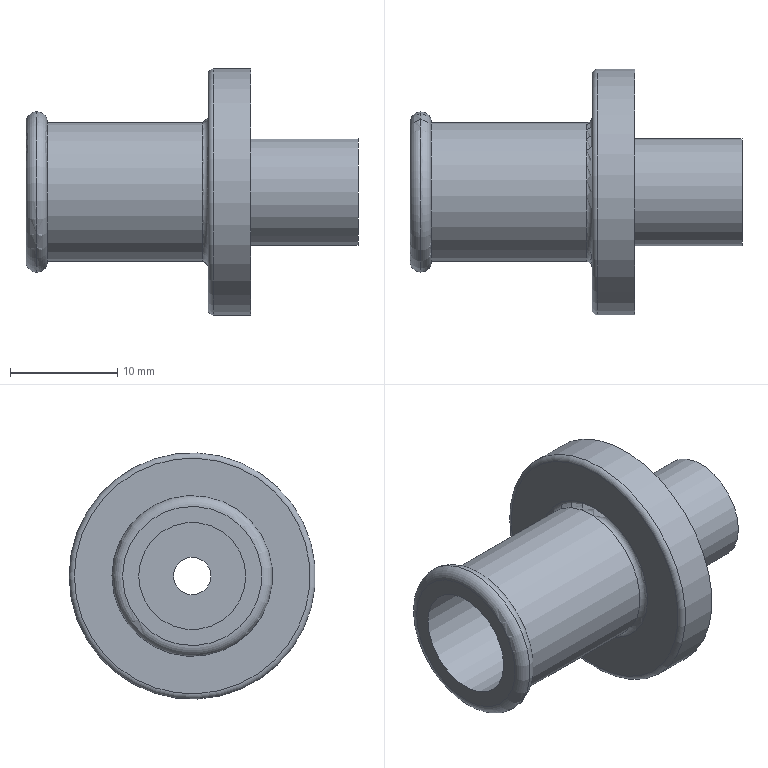Part | STEP file | 1-29.1 | 1 solid | 14 faces | box 31 x 23 x 23 mm | volume 3301 mm3 | cylinder 5 | plane 5 | torus 4 | commonest cylinder face diameters 10 x2 3.5 x1 13 x1 23 x1
STEP:
#1=CARTESIAN_POINT('',(0.,0.,0.));
#2=DIRECTION('',(0.,0.,1.));
#3=DIRECTION('',(1.,0.,0.));
#4=AXIS2_PLACEMENT_3D('',#1,#2,#3);
#5=CARTESIAN_POINT('',(15.,5.,0.));
#6=VERTEX_POINT('',#5);
#7=CARTESIAN_POINT('',(15.,0.,0.));
#8=DIRECTION('',(-1.,0.,0.));
#9=DIRECTION('',(0.,1.,0.));
#10=AXIS2_PLACEMENT_3D('',#7,#8,#9);
#11=CIRCLE('',#10,5.);
#12=CARTESIAN_POINT('',(-2.,0.,0.));
#13=DIRECTION('',(1.,0.,0.));
#14=DIRECTION('',(0.,1.,0.));
#15=AXIS2_PLACEMENT_3D('',#12,#13,#14);
#16=CYLINDRICAL_SURFACE('',#15,5.);
#17=CARTESIAN_POINT('',(6.283,17.));
#18=DIRECTION('',(-1.,0.));
#19=VECTOR('',#18,1.);
#20=LINE('',#17,#19);
#21=(GEOMETRIC_REPRESENTATION_CONTEXT(2)PARAMETRIC_REPRESENTATION_CONTEXT()REPRESENTATION_CONTEXT('',''));
#22=DEFINITIONAL_REPRESENTATION('',(#20),#21);
#23=PCURVE('',#16,#22);
#24=CARTESIAN_POINT('',(15.,-5.75,0.));
#25=DIRECTION('',(1.,0.,0.));
#26=DIRECTION('',(0.,0.,-1.));
#27=AXIS2_PLACEMENT_3D('',#24,#25,#26);
#28=PLANE('',#27);
#29=CARTESIAN_POINT('',(0.,10.75));
#30=CARTESIAN_POINT('',(8.66,10.75));
#31=CARTESIAN_POINT('',(4.33,3.25));
#32=CARTESIAN_POINT('',(0.,-4.25));
#33=CARTESIAN_POINT('',(-4.33,3.25));
#34=CARTESIAN_POINT('',(-8.66,10.75));
#35=CARTESIAN_POINT('',(0.,10.75));
#36=(BOUNDED_CURVE()B_SPLINE_CURVE(2,(#29,#30,#31,#32,#33,#34,#35),.UNSPECIFIED.,.T.,.F.)B_SPLINE_CURVE_WITH_KNOTS((1,2,2,2,2,1),(-2.094,0.,2.094,4.189,6.283,8.378),.UNSPECIFIED.)CURVE()GEOMETRIC_REPRESENTATION_ITEM()RATIONAL_B_SPLINE_CURVE((1.,0.5,1.,0.5,1.,0.5,1.))REPRESENTATION_ITEM(''));
#37=(GEOMETRIC_REPRESENTATION_CONTEXT(2)PARAMETRIC_REPRESENTATION_CONTEXT()REPRESENTATION_CONTEXT('',''));
#38=DEFINITIONAL_REPRESENTATION('',(#36),#37);
#39=PCURVE('',#28,#38);
#40=SURFACE_CURVE('',#11,(#23,#39),.PCURVE_S1.);
#41=EDGE_CURVE('',#6,#6,#40,.T.);
#42=ORIENTED_EDGE('',*,*,#41,.T.);
#43=CARTESIAN_POINT('',(-2.,5.,0.));
#44=VERTEX_POINT('',#43);
#45=CARTESIAN_POINT('',(15.,5.,0.));
#46=DIRECTION('',(-1.,0.,0.));
#47=VECTOR('',#46,1.);
#48=LINE('',#45,#47);
#49=CARTESIAN_POINT('',(0.,17.));
#50=DIRECTION('',(0.,-1.));
#51=VECTOR('',#50,1.);
#52=LINE('',#49,#51);
#53=(GEOMETRIC_REPRESENTATION_CONTEXT(2)PARAMETRIC_REPRESENTATION_CONTEXT()REPRESENTATION_CONTEXT('',''));
#54=DEFINITIONAL_REPRESENTATION('',(#52),#53);
#55=PCURVE('',#16,#54);
#56=CARTESIAN_POINT('',(6.283,17.));
#57=DIRECTION('',(0.,-1.));
#58=VECTOR('',#57,1.);
#59=LINE('',#56,#58);
#60=(GEOMETRIC_REPRESENTATION_CONTEXT(2)PARAMETRIC_REPRESENTATION_CONTEXT()REPRESENTATION_CONTEXT('',''));
#61=DEFINITIONAL_REPRESENTATION('',(#59),#60);
#62=PCURVE('',#16,#61);
#63=SEAM_CURVE('',#48,(#55,#62),.PCURVE_S1.);
#64=EDGE_CURVE('',#6,#44,#63,.T.);
#65=ORIENTED_EDGE('',*,*,#64,.T.);
#66=CARTESIAN_POINT('',(-2.,0.,0.));
#67=DIRECTION('',(-1.,0.,0.));
#68=DIRECTION('',(0.,1.,0.));
#69=AXIS2_PLACEMENT_3D('',#66,#67,#68);
#70=CIRCLE('',#69,5.);
#71=CARTESIAN_POINT('',(6.283,0.));
#72=DIRECTION('',(-1.,0.));
#73=VECTOR('',#72,1.);
#74=LINE('',#71,#73);
#75=(GEOMETRIC_REPRESENTATION_CONTEXT(2)PARAMETRIC_REPRESENTATION_CONTEXT()REPRESENTATION_CONTEXT('',''));
#76=DEFINITIONAL_REPRESENTATION('',(#74),#75);
#77=PCURVE('',#16,#76);
#78=CARTESIAN_POINT('',(-2.,-2.01,0.));
#79=DIRECTION('',(1.,0.,0.));
#80=DIRECTION('',(0.,0.,-1.));
#81=AXIS2_PLACEMENT_3D('',#78,#79,#80);
#82=PLANE('',#81);
#83=CARTESIAN_POINT('',(0.,7.01));
#84=CARTESIAN_POINT('',(8.66,7.01));
#85=CARTESIAN_POINT('',(4.33,-0.4904));
#86=CARTESIAN_POINT('',(0.,-7.99));
#87=CARTESIAN_POINT('',(-4.33,-0.4904));
#88=CARTESIAN_POINT('',(-8.66,7.01));
#89=CARTESIAN_POINT('',(0.,7.01));
#90=(BOUNDED_CURVE()B_SPLINE_CURVE(2,(#83,#84,#85,#86,#87,#88,#89),.UNSPECIFIED.,.T.,.F.)B_SPLINE_CURVE_WITH_KNOTS((1,2,2,2,2,1),(-2.094,0.,2.094,4.189,6.283,8.378),.UNSPECIFIED.)CURVE()GEOMETRIC_REPRESENTATION_ITEM()RATIONAL_B_SPLINE_CURVE((1.,0.5,1.,0.5,1.,0.5,1.))REPRESENTATION_ITEM(''));
#91=(GEOMETRIC_REPRESENTATION_CONTEXT(2)PARAMETRIC_REPRESENTATION_CONTEXT()REPRESENTATION_CONTEXT('',''));
#92=DEFINITIONAL_REPRESENTATION('',(#90),#91);
#93=PCURVE('',#82,#92);
#94=SURFACE_CURVE('',#70,(#77,#93),.PCURVE_S1.);
#95=EDGE_CURVE('',#44,#44,#94,.T.);
#96=ORIENTED_EDGE('',*,*,#95,.F.);
#97=ORIENTED_EDGE('',*,*,#64,.F.);
#98=EDGE_LOOP('',(#42,#65,#96,#97));
#99=FACE_BOUND('',#98,.F.);
#100=ADVANCED_FACE('',(#99),#16,.F.);
#101=CARTESIAN_POINT('',(19.,11.5,0.));
#102=VERTEX_POINT('',#101);
#103=CARTESIAN_POINT('',(19.,0.,0.));
#104=DIRECTION('',(1.,0.,0.));
#105=DIRECTION('',(0.,1.,0.));
#106=AXIS2_PLACEMENT_3D('',#103,#104,#105);
#107=CIRCLE('',#106,11.5);
#108=CARTESIAN_POINT('',(19.,-3.081,0.));
#109=DIRECTION('',(1.,0.,0.));
#110=DIRECTION('',(0.,0.,-1.));
#111=AXIS2_PLACEMENT_3D('',#108,#109,#110);
#112=PLANE('',#111);
#113=CARTESIAN_POINT('',(0.,3.081));
#114=DIRECTION('',(0.,1.));
#115=AXIS2_PLACEMENT_2D('',#113,#114);
#116=CIRCLE('',#115,11.5);
#117=(GEOMETRIC_REPRESENTATION_CONTEXT(2)PARAMETRIC_REPRESENTATION_CONTEXT()REPRESENTATION_CONTEXT('',''));
#118=DEFINITIONAL_REPRESENTATION('',(#116),#117);
#119=PCURVE('',#112,#118);
#120=CARTESIAN_POINT('',(15.,0.,0.));
#121=DIRECTION('',(1.,0.,0.));
#122=DIRECTION('',(0.,1.,0.));
#123=AXIS2_PLACEMENT_3D('',#120,#121,#122);
#124=CYLINDRICAL_SURFACE('',#123,11.5);
#125=CARTESIAN_POINT('',(0.,4.));
#126=DIRECTION('',(1.,0.));
#127=VECTOR('',#126,1.);
#128=LINE('',#125,#127);
#129=(GEOMETRIC_REPRESENTATION_CONTEXT(2)PARAMETRIC_REPRESENTATION_CONTEXT()REPRESENTATION_CONTEXT('',''));
#130=DEFINITIONAL_REPRESENTATION('',(#128),#129);
#131=PCURVE('',#124,#130);
#132=SURFACE_CURVE('',#107,(#119,#131),.PCURVE_S1.);
#133=EDGE_CURVE('',#102,#102,#132,.T.);
#134=ORIENTED_EDGE('',*,*,#133,.T.);
#135=EDGE_LOOP('',(#134));
#136=FACE_BOUND('',#135,.T.);
#137=CARTESIAN_POINT('',(19.,5.,0.));
#138=VERTEX_POINT('',#137);
#139=CARTESIAN_POINT('',(19.,0.,0.));
#140=DIRECTION('',(1.,0.,0.));
#141=DIRECTION('',(0.,1.,0.));
#142=AXIS2_PLACEMENT_3D('',#139,#140,#141);
#143=CIRCLE('',#142,5.);
#144=CARTESIAN_POINT('',(0.,3.081));
#145=DIRECTION('',(0.,1.));
#146=AXIS2_PLACEMENT_2D('',#144,#145);
#147=CIRCLE('',#146,5.);
#148=(GEOMETRIC_REPRESENTATION_CONTEXT(2)PARAMETRIC_REPRESENTATION_CONTEXT()REPRESENTATION_CONTEXT('',''));
#149=DEFINITIONAL_REPRESENTATION('',(#147),#148);
#150=PCURVE('',#112,#149);
#151=CARTESIAN_POINT('',(19.,0.,0.));
#152=DIRECTION('',(1.,0.,0.));
#153=DIRECTION('',(0.,1.,0.));
#154=AXIS2_PLACEMENT_3D('',#151,#152,#153);
#155=CYLINDRICAL_SURFACE('',#154,5.);
#156=CARTESIAN_POINT('',(0.,0.));
#157=DIRECTION('',(1.,0.));
#158=VECTOR('',#157,1.);
#159=LINE('',#156,#158);
#160=(GEOMETRIC_REPRESENTATION_CONTEXT(2)PARAMETRIC_REPRESENTATION_CONTEXT()REPRESENTATION_CONTEXT('',''));
#161=DEFINITIONAL_REPRESENTATION('',(#159),#160);
#162=PCURVE('',#155,#161);
#163=SURFACE_CURVE('',#143,(#150,#162),.PCURVE_S1.);
#164=EDGE_CURVE('',#138,#138,#163,.T.);
#165=ORIENTED_EDGE('',*,*,#164,.F.);
#166=EDGE_LOOP('',(#165));
#167=FACE_BOUND('',#166,.T.);
#168=ADVANCED_FACE('',(#136,#167),#112,.T.);
#169=ORIENTED_EDGE('',*,*,#164,.T.);
#170=CARTESIAN_POINT('',(29.,5.,0.));
#171=VERTEX_POINT('',#170);
#172=CARTESIAN_POINT('',(19.,5.,0.));
#173=DIRECTION('',(1.,0.,0.));
#174=VECTOR('',#173,1.);
#175=LINE('',#172,#174);
#176=CARTESIAN_POINT('',(6.283,0.));
#177=DIRECTION('',(0.,1.));
#178=VECTOR('',#177,1.);
#179=LINE('',#176,#178);
#180=(GEOMETRIC_REPRESENTATION_CONTEXT(2)PARAMETRIC_REPRESENTATION_CONTEXT()REPRESENTATION_CONTEXT('',''));
#181=DEFINITIONAL_REPRESENTATION('',(#179),#180);
#182=PCURVE('',#155,#181);
#183=CARTESIAN_POINT('',(0.,0.));
#184=DIRECTION('',(0.,1.));
#185=VECTOR('',#184,1.);
#186=LINE('',#183,#185);
#187=(GEOMETRIC_REPRESENTATION_CONTEXT(2)PARAMETRIC_REPRESENTATION_CONTEXT()REPRESENTATION_CONTEXT('',''));
#188=DEFINITIONAL_REPRESENTATION('',(#186),#187);
#189=PCURVE('',#155,#188);
#190=SEAM_CURVE('',#175,(#182,#189),.PCURVE_S1.);
#191=EDGE_CURVE('',#138,#171,#190,.T.);
#192=ORIENTED_EDGE('',*,*,#191,.T.);
#193=CARTESIAN_POINT('',(29.,0.,0.));
#194=DIRECTION('',(1.,0.,0.));
#195=DIRECTION('',(0.,1.,0.));
#196=AXIS2_PLACEMENT_3D('',#193,#194,#195);
#197=CIRCLE('',#196,5.);
#198=CARTESIAN_POINT('',(0.,10.));
#199=DIRECTION('',(1.,0.));
#200=VECTOR('',#199,1.);
#201=LINE('',#198,#200);
#202=(GEOMETRIC_REPRESENTATION_CONTEXT(2)PARAMETRIC_REPRESENTATION_CONTEXT()REPRESENTATION_CONTEXT('',''));
#203=DEFINITIONAL_REPRESENTATION('',(#201),#202);
#204=PCURVE('',#155,#203);
#205=CARTESIAN_POINT('',(29.,-1.34,0.));
#206=DIRECTION('',(1.,0.,0.));
#207=DIRECTION('',(0.,0.,-1.));
#208=AXIS2_PLACEMENT_3D('',#205,#206,#207);
#209=PLANE('',#208);
#210=CARTESIAN_POINT('',(0.,1.34));
#211=DIRECTION('',(0.,1.));
#212=AXIS2_PLACEMENT_2D('',#210,#211);
#213=CIRCLE('',#212,5.);
#214=(GEOMETRIC_REPRESENTATION_CONTEXT(2)PARAMETRIC_REPRESENTATION_CONTEXT()REPRESENTATION_CONTEXT('',''));
#215=DEFINITIONAL_REPRESENTATION('',(#213),#214);
#216=PCURVE('',#209,#215);
#217=SURFACE_CURVE('',#197,(#204,#216),.PCURVE_S1.);
#218=EDGE_CURVE('',#171,#171,#217,.T.);
#219=ORIENTED_EDGE('',*,*,#218,.F.);
#220=ORIENTED_EDGE('',*,*,#191,.F.);
#221=EDGE_LOOP('',(#169,#192,#219,#220));
#222=FACE_BOUND('',#221,.T.);
#223=ADVANCED_FACE('',(#222),#155,.T.);
#224=ORIENTED_EDGE('',*,*,#41,.F.);
#225=EDGE_LOOP('',(#224));
#226=FACE_BOUND('',#225,.F.);
#227=CARTESIAN_POINT('',(15.,1.75,0.));
#228=VERTEX_POINT('',#227);
#229=CARTESIAN_POINT('',(15.,0.,0.));
#230=DIRECTION('',(1.,0.,0.));
#231=DIRECTION('',(0.,1.,0.));
#232=AXIS2_PLACEMENT_3D('',#229,#230,#231);
#233=CIRCLE('',#232,1.75);
#234=CARTESIAN_POINT('',(0.,5.75));
#235=DIRECTION('',(0.,1.));
#236=AXIS2_PLACEMENT_2D('',#234,#235);
#237=CIRCLE('',#236,1.75);
#238=(GEOMETRIC_REPRESENTATION_CONTEXT(2)PARAMETRIC_REPRESENTATION_CONTEXT()REPRESENTATION_CONTEXT('',''));
#239=DEFINITIONAL_REPRESENTATION('',(#237),#238);
#240=PCURVE('',#28,#239);
#241=CARTESIAN_POINT('',(15.,0.,0.));
#242=DIRECTION('',(1.,0.,0.));
#243=DIRECTION('',(0.,1.,0.));
#244=AXIS2_PLACEMENT_3D('',#241,#242,#243);
#245=CYLINDRICAL_SURFACE('',#244,1.75);
#246=CARTESIAN_POINT('',(0.,0.));
#247=DIRECTION('',(1.,0.));
#248=VECTOR('',#247,1.);
#249=LINE('',#246,#248);
#250=(GEOMETRIC_REPRESENTATION_CONTEXT(2)PARAMETRIC_REPRESENTATION_CONTEXT()REPRESENTATION_CONTEXT('',''));
#251=DEFINITIONAL_REPRESENTATION('',(#249),#250);
#252=PCURVE('',#245,#251);
#253=SURFACE_CURVE('',#233,(#240,#252),.PCURVE_S1.);
#254=EDGE_CURVE('',#228,#228,#253,.T.);
#255=ORIENTED_EDGE('',*,*,#254,.F.);
#256=EDGE_LOOP('',(#255));
#257=FACE_BOUND('',#256,.F.);
#258=ADVANCED_FACE('',(#226,#257),#28,.F.);
#259=ORIENTED_EDGE('',*,*,#218,.T.);
#260=EDGE_LOOP('',(#259));
#261=FACE_BOUND('',#260,.T.);
#262=CARTESIAN_POINT('',(29.,1.75,0.));
#263=VERTEX_POINT('',#262);
#264=CARTESIAN_POINT('',(29.,0.,0.));
#265=DIRECTION('',(1.,0.,0.));
#266=DIRECTION('',(0.,1.,0.));
#267=AXIS2_PLACEMENT_3D('',#264,#265,#266);
#268=CIRCLE('',#267,1.75);
#269=CARTESIAN_POINT('',(0.,1.34));
#270=DIRECTION('',(0.,1.));
#271=AXIS2_PLACEMENT_2D('',#269,#270);
#272=CIRCLE('',#271,1.75);
#273=(GEOMETRIC_REPRESENTATION_CONTEXT(2)PARAMETRIC_REPRESENTATION_CONTEXT()REPRESENTATION_CONTEXT('',''));
#274=DEFINITIONAL_REPRESENTATION('',(#272),#273);
#275=PCURVE('',#209,#274);
#276=CARTESIAN_POINT('',(0.,14.));
#277=DIRECTION('',(1.,0.));
#278=VECTOR('',#277,1.);
#279=LINE('',#276,#278);
#280=(GEOMETRIC_REPRESENTATION_CONTEXT(2)PARAMETRIC_REPRESENTATION_CONTEXT()REPRESENTATION_CONTEXT('',''));
#281=DEFINITIONAL_REPRESENTATION('',(#279),#280);
#282=PCURVE('',#245,#281);
#283=SURFACE_CURVE('',#268,(#275,#282),.PCURVE_S1.);
#284=EDGE_CURVE('',#263,#263,#283,.T.);
#285=ORIENTED_EDGE('',*,*,#284,.F.);
#286=EDGE_LOOP('',(#285));
#287=FACE_BOUND('',#286,.T.);
#288=ADVANCED_FACE('',(#261,#287),#209,.T.);
#289=ORIENTED_EDGE('',*,*,#254,.T.);
#290=CARTESIAN_POINT('',(15.,1.75,0.));
#291=DIRECTION('',(1.,0.,0.));
#292=VECTOR('',#291,1.);
#293=LINE('',#290,#292);
#294=CARTESIAN_POINT('',(6.283,0.));
#295=DIRECTION('',(0.,1.));
#296=VECTOR('',#295,1.);
#297=LINE('',#294,#296);
#298=(GEOMETRIC_REPRESENTATION_CONTEXT(2)PARAMETRIC_REPRESENTATION_CONTEXT()REPRESENTATION_CONTEXT('',''));
#299=DEFINITIONAL_REPRESENTATION('',(#297),#298);
#300=PCURVE('',#245,#299);
#301=CARTESIAN_POINT('',(0.,0.));
#302=DIRECTION('',(0.,1.));
#303=VECTOR('',#302,1.);
#304=LINE('',#301,#303);
#305=(GEOMETRIC_REPRESENTATION_CONTEXT(2)PARAMETRIC_REPRESENTATION_CONTEXT()REPRESENTATION_CONTEXT('',''));
#306=DEFINITIONAL_REPRESENTATION('',(#304),#305);
#307=PCURVE('',#245,#306);
#308=SEAM_CURVE('',#293,(#300,#307),.PCURVE_S1.);
#309=EDGE_CURVE('',#228,#263,#308,.T.);
#310=ORIENTED_EDGE('',*,*,#309,.T.);
#311=ORIENTED_EDGE('',*,*,#284,.F.);
#312=ORIENTED_EDGE('',*,*,#309,.F.);
#313=EDGE_LOOP('',(#289,#310,#311,#312));
#314=FACE_BOUND('',#313,.F.);
#315=ADVANCED_FACE('',(#314),#245,.F.);
#316=CARTESIAN_POINT('',(-2.,6.5,0.));
#317=VERTEX_POINT('',#316);
#318=CARTESIAN_POINT('',(-2.,0.,0.));
#319=DIRECTION('',(1.,0.,0.));
#320=DIRECTION('',(0.,1.,0.));
#321=AXIS2_PLACEMENT_3D('',#318,#319,#320);
#322=CIRCLE('',#321,6.5);
#323=CARTESIAN_POINT('',(0.,2.01));
#324=DIRECTION('',(0.,1.));
#325=AXIS2_PLACEMENT_2D('',#323,#324);
#326=CIRCLE('',#325,6.5);
#327=(GEOMETRIC_REPRESENTATION_CONTEXT(2)PARAMETRIC_REPRESENTATION_CONTEXT()REPRESENTATION_CONTEXT('',''));
#328=DEFINITIONAL_REPRESENTATION('',(#326),#327);
#329=PCURVE('',#82,#328);
#330=CARTESIAN_POINT('',(-1.,0.,0.));
#331=DIRECTION('',(-1.,0.,0.));
#332=DIRECTION('',(0.,1.,0.));
#333=AXIS2_PLACEMENT_3D('',#330,#331,#332);
#334=TOROIDAL_SURFACE('',#333,6.5,1.);
#335=CARTESIAN_POINT('',(6.283,1.571));
#336=DIRECTION('',(-1.,0.));
#337=VECTOR('',#336,1.);
#338=LINE('',#335,#337);
#339=(GEOMETRIC_REPRESENTATION_CONTEXT(2)PARAMETRIC_REPRESENTATION_CONTEXT()REPRESENTATION_CONTEXT('',''));
#340=DEFINITIONAL_REPRESENTATION('',(#338),#339);
#341=PCURVE('',#334,#340);
#342=SURFACE_CURVE('',#322,(#329,#341),.PCURVE_S1.);
#343=EDGE_CURVE('',#317,#317,#342,.T.);
#344=ORIENTED_EDGE('',*,*,#343,.T.);
#345=EDGE_LOOP('',(#344));
#346=FACE_BOUND('',#345,.F.);
#347=ORIENTED_EDGE('',*,*,#95,.T.);
#348=EDGE_LOOP('',(#347));
#349=FACE_BOUND('',#348,.F.);
#350=ADVANCED_FACE('',(#346,#349),#82,.F.);
#351=CARTESIAN_POINT('',(0.,6.5,0.));
#352=VERTEX_POINT('',#351);
#353=CARTESIAN_POINT('',(0.,0.,0.));
#354=DIRECTION('',(1.,0.,0.));
#355=DIRECTION('',(0.,1.,0.));
#356=AXIS2_PLACEMENT_3D('',#353,#354,#355);
#357=CIRCLE('',#356,6.5);
#358=CARTESIAN_POINT('',(-1.,0.,0.));
#359=DIRECTION('',(-1.,0.,0.));
#360=DIRECTION('',(0.,1.,0.));
#361=AXIS2_PLACEMENT_3D('',#358,#359,#360);
#362=TOROIDAL_SURFACE('',#361,6.5,1.);
#363=CARTESIAN_POINT('',(6.283,4.712));
#364=DIRECTION('',(-1.,0.));
#365=VECTOR('',#364,1.);
#366=LINE('',#363,#365);
#367=(GEOMETRIC_REPRESENTATION_CONTEXT(2)PARAMETRIC_REPRESENTATION_CONTEXT()REPRESENTATION_CONTEXT('',''));
#368=DEFINITIONAL_REPRESENTATION('',(#366),#367);
#369=PCURVE('',#362,#368);
#370=CARTESIAN_POINT('',(0.,0.,0.));
#371=DIRECTION('',(1.,0.,0.));
#372=DIRECTION('',(0.,1.,0.));
#373=AXIS2_PLACEMENT_3D('',#370,#371,#372);
#374=CYLINDRICAL_SURFACE('',#373,6.5);
#375=CARTESIAN_POINT('',(0.,0.));
#376=DIRECTION('',(1.,0.));
#377=VECTOR('',#376,1.);
#378=LINE('',#375,#377);
#379=(GEOMETRIC_REPRESENTATION_CONTEXT(2)PARAMETRIC_REPRESENTATION_CONTEXT()REPRESENTATION_CONTEXT('',''));
#380=DEFINITIONAL_REPRESENTATION('',(#378),#379);
#381=PCURVE('',#374,#380);
#382=SURFACE_CURVE('',#357,(#369,#381),.PCURVE_S1.);
#383=EDGE_CURVE('',#352,#352,#382,.T.);
#384=ORIENTED_EDGE('',*,*,#383,.F.);
#385=CARTESIAN_POINT('',(-1.,7.5,0.));
#386=VERTEX_POINT('',#385);
#387=CARTESIAN_POINT('',(-1.,6.5,0.));
#388=DIRECTION('',(0.,0.,1.));
#389=DIRECTION('',(1.,0.,0.));
#390=AXIS2_PLACEMENT_3D('',#387,#388,#389);
#391=CIRCLE('',#390,1.);
#392=CARTESIAN_POINT('',(6.283,4.712));
#393=DIRECTION('',(0.,1.));
#394=VECTOR('',#393,1.);
#395=LINE('',#392,#394);
#396=(GEOMETRIC_REPRESENTATION_CONTEXT(2)PARAMETRIC_REPRESENTATION_CONTEXT()REPRESENTATION_CONTEXT('',''));
#397=DEFINITIONAL_REPRESENTATION('',(#395),#396);
#398=PCURVE('',#362,#397);
#399=CARTESIAN_POINT('',(0.,4.712));
#400=DIRECTION('',(0.,1.));
#401=VECTOR('',#400,1.);
#402=LINE('',#399,#401);
#403=(GEOMETRIC_REPRESENTATION_CONTEXT(2)PARAMETRIC_REPRESENTATION_CONTEXT()REPRESENTATION_CONTEXT('',''));
#404=DEFINITIONAL_REPRESENTATION('',(#402),#403);
#405=PCURVE('',#362,#404);
#406=SEAM_CURVE('',#391,(#398,#405),.PCURVE_S1.);
#407=EDGE_CURVE('',#352,#386,#406,.T.);
#408=ORIENTED_EDGE('',*,*,#407,.T.);
#409=CARTESIAN_POINT('',(-1.,0.,0.));
#410=DIRECTION('',(1.,0.,0.));
#411=DIRECTION('',(0.,1.,0.));
#412=AXIS2_PLACEMENT_3D('',#409,#410,#411);
#413=CIRCLE('',#412,7.5);
#414=CARTESIAN_POINT('',(6.283,6.283));
#415=DIRECTION('',(-1.,0.));
#416=VECTOR('',#415,1.);
#417=LINE('',#414,#416);
#418=(GEOMETRIC_REPRESENTATION_CONTEXT(2)PARAMETRIC_REPRESENTATION_CONTEXT()REPRESENTATION_CONTEXT('',''));
#419=DEFINITIONAL_REPRESENTATION('',(#417),#418);
#420=PCURVE('',#362,#419);
#421=CARTESIAN_POINT('',(6.283,0.));
#422=DIRECTION('',(-1.,0.));
#423=VECTOR('',#422,1.);
#424=LINE('',#421,#423);
#425=(GEOMETRIC_REPRESENTATION_CONTEXT(2)PARAMETRIC_REPRESENTATION_CONTEXT()REPRESENTATION_CONTEXT('',''));
#426=DEFINITIONAL_REPRESENTATION('',(#424),#425);
#427=PCURVE('',#334,#426);
#428=SURFACE_CURVE('',#413,(#420,#427),.PCURVE_S1.);
#429=EDGE_CURVE('',#386,#386,#428,.T.);
#430=ORIENTED_EDGE('',*,*,#429,.T.);
#431=ORIENTED_EDGE('',*,*,#407,.F.);
#432=EDGE_LOOP('',(#384,#408,#430,#431));
#433=FACE_BOUND('',#432,.T.);
#434=ADVANCED_FACE('',(#433),#362,.T.);
#435=CARTESIAN_POINT('',(-1.,6.5,0.));
#436=DIRECTION('',(0.,0.,-1.));
#437=DIRECTION('',(-1.,0.,0.));
#438=AXIS2_PLACEMENT_3D('',#435,#436,#437);
#439=CIRCLE('',#438,1.);
#440=CARTESIAN_POINT('',(0.,1.571));
#441=DIRECTION('',(0.,-1.));
#442=VECTOR('',#441,1.);
#443=LINE('',#440,#442);
#444=(GEOMETRIC_REPRESENTATION_CONTEXT(2)PARAMETRIC_REPRESENTATION_CONTEXT()REPRESENTATION_CONTEXT('',''));
#445=DEFINITIONAL_REPRESENTATION('',(#443),#444);
#446=PCURVE('',#334,#445);
#447=CARTESIAN_POINT('',(6.283,1.571));
#448=DIRECTION('',(0.,-1.));
#449=VECTOR('',#448,1.);
#450=LINE('',#447,#449);
#451=(GEOMETRIC_REPRESENTATION_CONTEXT(2)PARAMETRIC_REPRESENTATION_CONTEXT()REPRESENTATION_CONTEXT('',''));
#452=DEFINITIONAL_REPRESENTATION('',(#450),#451);
#453=PCURVE('',#334,#452);
#454=SEAM_CURVE('',#439,(#446,#453),.PCURVE_S1.);
#455=EDGE_CURVE('',#317,#386,#454,.T.);
#456=ORIENTED_EDGE('',*,*,#455,.T.);
#457=ORIENTED_EDGE('',*,*,#429,.F.);
#458=ORIENTED_EDGE('',*,*,#455,.F.);
#459=ORIENTED_EDGE('',*,*,#343,.T.);
#460=EDGE_LOOP('',(#456,#457,#458,#459));
#461=FACE_BOUND('',#460,.T.);
#462=ADVANCED_FACE('',(#461),#334,.T.);
#463=ORIENTED_EDGE('',*,*,#383,.T.);
#464=CARTESIAN_POINT('',(14.5,6.5,0.));
#465=VERTEX_POINT('',#464);
#466=CARTESIAN_POINT('',(0.,6.5,0.));
#467=DIRECTION('',(1.,0.,0.));
#468=VECTOR('',#467,1.);
#469=LINE('',#466,#468);
#470=CARTESIAN_POINT('',(6.283,0.));
#471=DIRECTION('',(0.,1.));
#472=VECTOR('',#471,1.);
#473=LINE('',#470,#472);
#474=(GEOMETRIC_REPRESENTATION_CONTEXT(2)PARAMETRIC_REPRESENTATION_CONTEXT()REPRESENTATION_CONTEXT('',''));
#475=DEFINITIONAL_REPRESENTATION('',(#473),#474);
#476=PCURVE('',#374,#475);
#477=CARTESIAN_POINT('',(0.,0.));
#478=DIRECTION('',(0.,1.));
#479=VECTOR('',#478,1.);
#480=LINE('',#477,#479);
#481=(GEOMETRIC_REPRESENTATION_CONTEXT(2)PARAMETRIC_REPRESENTATION_CONTEXT()REPRESENTATION_CONTEXT('',''));
#482=DEFINITIONAL_REPRESENTATION('',(#480),#481);
#483=PCURVE('',#374,#482);
#484=SEAM_CURVE('',#469,(#476,#483),.PCURVE_S1.);
#485=EDGE_CURVE('',#352,#465,#484,.T.);
#486=ORIENTED_EDGE('',*,*,#485,.T.);
#487=CARTESIAN_POINT('',(14.5,0.,0.));
#488=DIRECTION('',(-1.,0.,0.));
#489=DIRECTION('',(0.,1.,0.));
#490=AXIS2_PLACEMENT_3D('',#487,#488,#489);
#491=CIRCLE('',#490,6.5);
#492=CARTESIAN_POINT('',(6.283,14.5));
#493=DIRECTION('',(-1.,0.));
#494=VECTOR('',#493,1.);
#495=LINE('',#492,#494);
#496=(GEOMETRIC_REPRESENTATION_CONTEXT(2)PARAMETRIC_REPRESENTATION_CONTEXT()REPRESENTATION_CONTEXT('',''));
#497=DEFINITIONAL_REPRESENTATION('',(#495),#496);
#498=PCURVE('',#374,#497);
#499=CARTESIAN_POINT('',(14.5,0.,0.));
#500=DIRECTION('',(1.,0.,0.));
#501=DIRECTION('',(0.,1.,0.));
#502=AXIS2_PLACEMENT_3D('',#499,#500,#501);
#503=TOROIDAL_SURFACE('',#502,7.,0.5);
#504=CARTESIAN_POINT('',(6.283,3.142));
#505=DIRECTION('',(-1.,0.));
#506=VECTOR('',#505,1.);
#507=LINE('',#504,#506);
#508=(GEOMETRIC_REPRESENTATION_CONTEXT(2)PARAMETRIC_REPRESENTATION_CONTEXT()REPRESENTATION_CONTEXT('',''));
#509=DEFINITIONAL_REPRESENTATION('',(#507),#508);
#510=PCURVE('',#503,#509);
#511=SURFACE_CURVE('',#491,(#498,#510),.PCURVE_S1.);
#512=EDGE_CURVE('',#465,#465,#511,.T.);
#513=ORIENTED_EDGE('',*,*,#512,.T.);
#514=ORIENTED_EDGE('',*,*,#485,.F.);
#515=EDGE_LOOP('',(#463,#486,#513,#514));
#516=FACE_BOUND('',#515,.T.);
#517=ADVANCED_FACE('',(#516),#374,.T.);
#518=CARTESIAN_POINT('',(15.,11.,0.));
#519=VERTEX_POINT('',#518);
#520=CARTESIAN_POINT('',(15.,0.,0.));
#521=DIRECTION('',(-1.,0.,0.));
#522=DIRECTION('',(0.,1.,0.));
#523=AXIS2_PLACEMENT_3D('',#520,#521,#522);
#524=CIRCLE('',#523,11.);
#525=CARTESIAN_POINT('',(15.,-5.75,0.));
#526=DIRECTION('',(1.,0.,0.));
#527=DIRECTION('',(0.,0.,-1.));
#528=AXIS2_PLACEMENT_3D('',#525,#526,#527);
#529=PLANE('',#528);
#530=CARTESIAN_POINT('',(0.,16.75));
#531=CARTESIAN_POINT('',(19.053,16.75));
#532=CARTESIAN_POINT('',(9.526,0.25));
#533=CARTESIAN_POINT('',(0.,-16.25));
#534=CARTESIAN_POINT('',(-9.526,0.25));
#535=CARTESIAN_POINT('',(-19.053,16.75));
#536=CARTESIAN_POINT('',(0.,16.75));
#537=(BOUNDED_CURVE()B_SPLINE_CURVE(2,(#530,#531,#532,#533,#534,#535,#536),.UNSPECIFIED.,.T.,.F.)B_SPLINE_CURVE_WITH_KNOTS((1,2,2,2,2,1),(-2.094,0.,2.094,4.189,6.283,8.378),.UNSPECIFIED.)CURVE()GEOMETRIC_REPRESENTATION_ITEM()RATIONAL_B_SPLINE_CURVE((1.,0.5,1.,0.5,1.,0.5,1.))REPRESENTATION_ITEM(''));
#538=(GEOMETRIC_REPRESENTATION_CONTEXT(2)PARAMETRIC_REPRESENTATION_CONTEXT()REPRESENTATION_CONTEXT('',''));
#539=DEFINITIONAL_REPRESENTATION('',(#537),#538);
#540=PCURVE('',#529,#539);
#541=CARTESIAN_POINT('',(15.5,0.,0.));
#542=DIRECTION('',(1.,0.,0.));
#543=DIRECTION('',(0.,1.,0.));
#544=AXIS2_PLACEMENT_3D('',#541,#542,#543);
#545=TOROIDAL_SURFACE('',#544,11.,0.5);
#546=CARTESIAN_POINT('',(6.283,4.712));
#547=DIRECTION('',(-1.,0.));
#548=VECTOR('',#547,1.);
#549=LINE('',#546,#548);
#550=(GEOMETRIC_REPRESENTATION_CONTEXT(2)PARAMETRIC_REPRESENTATION_CONTEXT()REPRESENTATION_CONTEXT('',''));
#551=DEFINITIONAL_REPRESENTATION('',(#549),#550);
#552=PCURVE('',#545,#551);
#553=SURFACE_CURVE('',#524,(#540,#552),.PCURVE_S1.);
#554=EDGE_CURVE('',#519,#519,#553,.T.);
#555=ORIENTED_EDGE('',*,*,#554,.F.);
#556=EDGE_LOOP('',(#555));
#557=FACE_BOUND('',#556,.F.);
#558=CARTESIAN_POINT('',(15.,7.,0.));
#559=VERTEX_POINT('',#558);
#560=CARTESIAN_POINT('',(15.,0.,0.));
#561=DIRECTION('',(-1.,0.,0.));
#562=DIRECTION('',(0.,1.,0.));
#563=AXIS2_PLACEMENT_3D('',#560,#561,#562);
#564=CIRCLE('',#563,7.);
#565=CARTESIAN_POINT('',(0.,12.75));
#566=CARTESIAN_POINT('',(12.124,12.75));
#567=CARTESIAN_POINT('',(6.062,2.25));
#568=CARTESIAN_POINT('',(0.,-8.25));
#569=CARTESIAN_POINT('',(-6.062,2.25));
#570=CARTESIAN_POINT('',(-12.124,12.75));
#571=CARTESIAN_POINT('',(0.,12.75));
#572=(BOUNDED_CURVE()B_SPLINE_CURVE(2,(#565,#566,#567,#568,#569,#570,#571),.UNSPECIFIED.,.T.,.F.)B_SPLINE_CURVE_WITH_KNOTS((1,2,2,2,2,1),(-2.094,0.,2.094,4.189,6.283,8.378),.UNSPECIFIED.)CURVE()GEOMETRIC_REPRESENTATION_ITEM()RATIONAL_B_SPLINE_CURVE((1.,0.5,1.,0.5,1.,0.5,1.))REPRESENTATION_ITEM(''));
#573=(GEOMETRIC_REPRESENTATION_CONTEXT(2)PARAMETRIC_REPRESENTATION_CONTEXT()REPRESENTATION_CONTEXT('',''));
#574=DEFINITIONAL_REPRESENTATION('',(#572),#573);
#575=PCURVE('',#529,#574);
#576=CARTESIAN_POINT('',(6.283,1.571));
#577=DIRECTION('',(-1.,0.));
#578=VECTOR('',#577,1.);
#579=LINE('',#576,#578);
#580=(GEOMETRIC_REPRESENTATION_CONTEXT(2)PARAMETRIC_REPRESENTATION_CONTEXT()REPRESENTATION_CONTEXT('',''));
#581=DEFINITIONAL_REPRESENTATION('',(#579),#580);
#582=PCURVE('',#503,#581);
#583=SURFACE_CURVE('',#564,(#575,#582),.PCURVE_S1.);
#584=EDGE_CURVE('',#559,#559,#583,.T.);
#585=ORIENTED_EDGE('',*,*,#584,.T.);
#586=EDGE_LOOP('',(#585));
#587=FACE_BOUND('',#586,.F.);
#588=ADVANCED_FACE('',(#557,#587),#529,.F.);
#589=ORIENTED_EDGE('',*,*,#133,.F.);
#590=CARTESIAN_POINT('',(15.5,11.5,0.));
#591=VERTEX_POINT('',#590);
#592=CARTESIAN_POINT('',(15.5,11.5,0.));
#593=DIRECTION('',(1.,0.,0.));
#594=VECTOR('',#593,1.);
#595=LINE('',#592,#594);
#596=CARTESIAN_POINT('',(0.,0.5));
#597=DIRECTION('',(0.,1.));
#598=VECTOR('',#597,1.);
#599=LINE('',#596,#598);
#600=(GEOMETRIC_REPRESENTATION_CONTEXT(2)PARAMETRIC_REPRESENTATION_CONTEXT()REPRESENTATION_CONTEXT('',''));
#601=DEFINITIONAL_REPRESENTATION('',(#599),#600);
#602=PCURVE('',#124,#601);
#603=CARTESIAN_POINT('',(6.283,0.5));
#604=DIRECTION('',(0.,1.));
#605=VECTOR('',#604,1.);
#606=LINE('',#603,#605);
#607=(GEOMETRIC_REPRESENTATION_CONTEXT(2)PARAMETRIC_REPRESENTATION_CONTEXT()REPRESENTATION_CONTEXT('',''));
#608=DEFINITIONAL_REPRESENTATION('',(#606),#607);
#609=PCURVE('',#124,#608);
#610=SEAM_CURVE('',#595,(#602,#609),.PCURVE_S1.);
#611=EDGE_CURVE('',#591,#102,#610,.T.);
#612=ORIENTED_EDGE('',*,*,#611,.F.);
#613=CARTESIAN_POINT('',(15.5,0.,0.));
#614=DIRECTION('',(-1.,0.,0.));
#615=DIRECTION('',(0.,1.,0.));
#616=AXIS2_PLACEMENT_3D('',#613,#614,#615);
#617=CIRCLE('',#616,11.5);
#618=CARTESIAN_POINT('',(6.283,0.5));
#619=DIRECTION('',(-1.,0.));
#620=VECTOR('',#619,1.);
#621=LINE('',#618,#620);
#622=(GEOMETRIC_REPRESENTATION_CONTEXT(2)PARAMETRIC_REPRESENTATION_CONTEXT()REPRESENTATION_CONTEXT('',''));
#623=DEFINITIONAL_REPRESENTATION('',(#621),#622);
#624=PCURVE('',#124,#623);
#625=CARTESIAN_POINT('',(6.283,6.283));
#626=DIRECTION('',(-1.,0.));
#627=VECTOR('',#626,1.);
#628=LINE('',#625,#627);
#629=(GEOMETRIC_REPRESENTATION_CONTEXT(2)PARAMETRIC_REPRESENTATION_CONTEXT()REPRESENTATION_CONTEXT('',''));
#630=DEFINITIONAL_REPRESENTATION('',(#628),#629);
#631=PCURVE('',#545,#630);
#632=SURFACE_CURVE('',#617,(#624,#631),.PCURVE_S1.);
#633=EDGE_CURVE('',#591,#591,#632,.T.);
#634=ORIENTED_EDGE('',*,*,#633,.F.);
#635=ORIENTED_EDGE('',*,*,#611,.T.);
#636=EDGE_LOOP('',(#589,#612,#634,#635));
#637=FACE_BOUND('',#636,.T.);
#638=ADVANCED_FACE('',(#637),#124,.T.);
#639=ORIENTED_EDGE('',*,*,#584,.F.);
#640=CARTESIAN_POINT('',(14.5,7.,0.));
#641=DIRECTION('',(0.,0.,1.));
#642=DIRECTION('',(0.,-1.,0.));
#643=AXIS2_PLACEMENT_3D('',#640,#641,#642);
#644=CIRCLE('',#643,0.5);
#645=CARTESIAN_POINT('',(6.283,3.142));
#646=DIRECTION('',(0.,-1.));
#647=VECTOR('',#646,1.);
#648=LINE('',#645,#647);
#649=(GEOMETRIC_REPRESENTATION_CONTEXT(2)PARAMETRIC_REPRESENTATION_CONTEXT()REPRESENTATION_CONTEXT('',''));
#650=DEFINITIONAL_REPRESENTATION('',(#648),#649);
#651=PCURVE('',#503,#650);
#652=CARTESIAN_POINT('',(0.,3.142));
#653=DIRECTION('',(0.,-1.));
#654=VECTOR('',#653,1.);
#655=LINE('',#652,#654);
#656=(GEOMETRIC_REPRESENTATION_CONTEXT(2)PARAMETRIC_REPRESENTATION_CONTEXT()REPRESENTATION_CONTEXT('',''));
#657=DEFINITIONAL_REPRESENTATION('',(#655),#656);
#658=PCURVE('',#503,#657);
#659=SEAM_CURVE('',#644,(#651,#658),.PCURVE_S1.);
#660=EDGE_CURVE('',#465,#559,#659,.T.);
#661=ORIENTED_EDGE('',*,*,#660,.F.);
#662=ORIENTED_EDGE('',*,*,#512,.T.);
#663=ORIENTED_EDGE('',*,*,#660,.T.);
#664=EDGE_LOOP('',(#639,#661,#662,#663));
#665=FACE_BOUND('',#664,.F.);
#666=ADVANCED_FACE('',(#665),#503,.F.);
#667=ORIENTED_EDGE('',*,*,#554,.F.);
#668=CARTESIAN_POINT('',(15.5,11.,0.));
#669=DIRECTION('',(0.,0.,-1.));
#670=DIRECTION('',(-1.,0.,0.));
#671=AXIS2_PLACEMENT_3D('',#668,#669,#670);
#672=CIRCLE('',#671,0.5);
#673=CARTESIAN_POINT('',(6.283,4.712));
#674=DIRECTION('',(0.,1.));
#675=VECTOR('',#674,1.);
#676=LINE('',#673,#675);
#677=(GEOMETRIC_REPRESENTATION_CONTEXT(2)PARAMETRIC_REPRESENTATION_CONTEXT()REPRESENTATION_CONTEXT('',''));
#678=DEFINITIONAL_REPRESENTATION('',(#676),#677);
#679=PCURVE('',#545,#678);
#680=CARTESIAN_POINT('',(0.,4.712));
#681=DIRECTION('',(0.,1.));
#682=VECTOR('',#681,1.);
#683=LINE('',#680,#682);
#684=(GEOMETRIC_REPRESENTATION_CONTEXT(2)PARAMETRIC_REPRESENTATION_CONTEXT()REPRESENTATION_CONTEXT('',''));
#685=DEFINITIONAL_REPRESENTATION('',(#683),#684);
#686=PCURVE('',#545,#685);
#687=SEAM_CURVE('',#672,(#679,#686),.PCURVE_S1.);
#688=EDGE_CURVE('',#519,#591,#687,.T.);
#689=ORIENTED_EDGE('',*,*,#688,.T.);
#690=ORIENTED_EDGE('',*,*,#633,.T.);
#691=ORIENTED_EDGE('',*,*,#688,.F.);
#692=EDGE_LOOP('',(#667,#689,#690,#691));
#693=FACE_BOUND('',#692,.T.);
#694=ADVANCED_FACE('',(#693),#545,.T.);
#695=CLOSED_SHELL('',(#100,#168,#223,#258,#288,#315,#350,#434,#462,#517,#588,#638,#666,#694));
#696=MANIFOLD_SOLID_BREP('',#695);
#697=(LENGTH_UNIT()NAMED_UNIT(*)SI_UNIT(.MILLI.,.METRE.));
#698=UNCERTAINTY_MEASURE_WITH_UNIT(LENGTH_MEASURE(0.0000001),#697,'','');
#699=(NAMED_UNIT(*)PLANE_ANGLE_UNIT()SI_UNIT($,.RADIAN.));
#700=(NAMED_UNIT(*)SI_UNIT($,.STERADIAN.)SOLID_ANGLE_UNIT());
#701=(GEOMETRIC_REPRESENTATION_CONTEXT(3)GLOBAL_UNCERTAINTY_ASSIGNED_CONTEXT((#698))GLOBAL_UNIT_ASSIGNED_CONTEXT((#697,#699,#700))REPRESENTATION_CONTEXT('',''));
#702=ADVANCED_BREP_SHAPE_REPRESENTATION('',(#4,#696),#701);